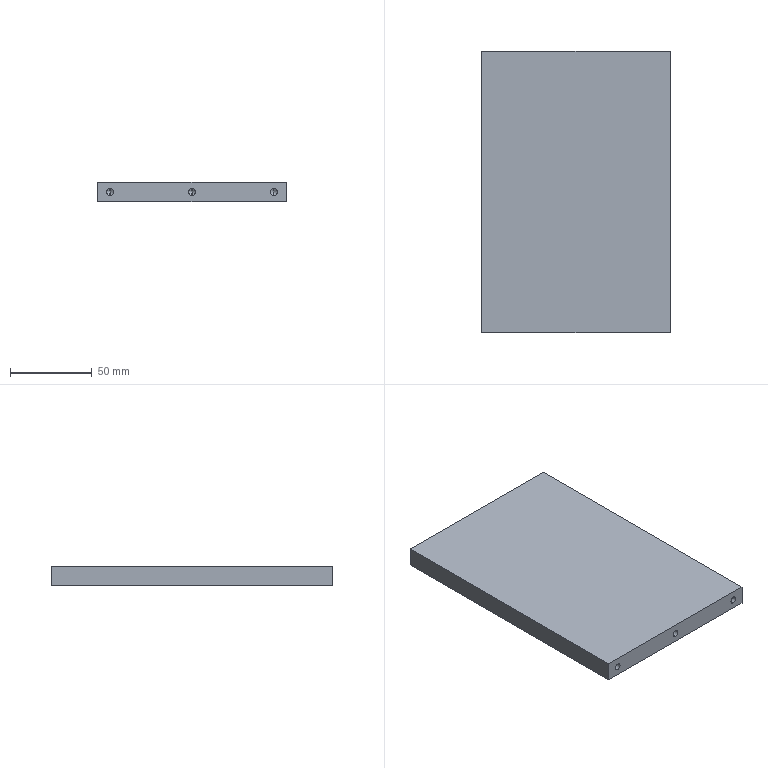Part | STEP file | PN_0003 Mount electronic clip support plate B | 1 solid | 26 faces | box 115 x 172 x 12 mm | volume 236361 mm3 | cylinder 10 | cone 10 | plane 6 | commonest cylinder face diameters 4.2 x10